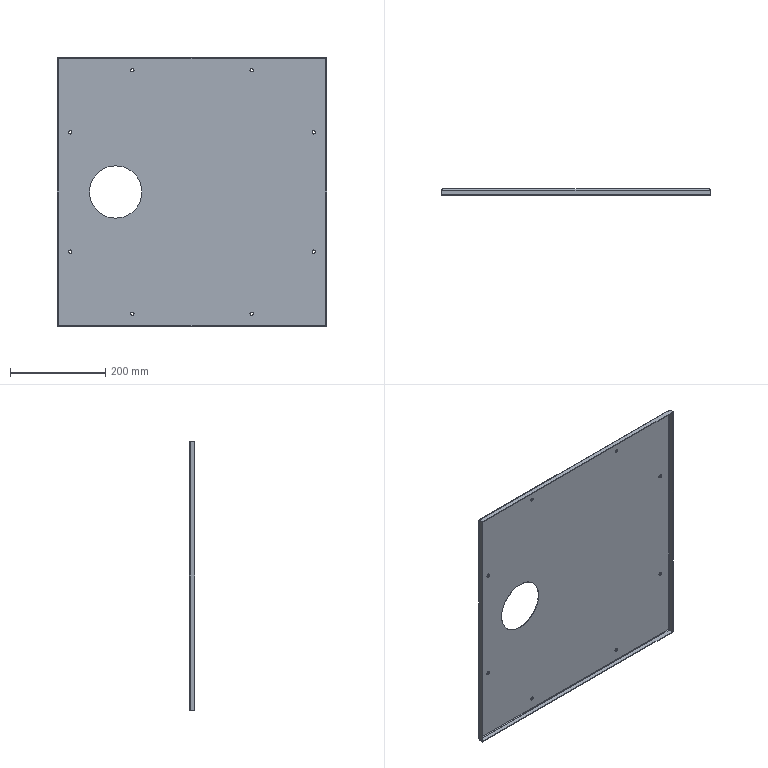Part | STEP file | 1 solid | 64 faces | box 565 x 12 x 565 mm | volume 496282 mm3 | plane 38 | cylinder 26 | commonest cylinder face diameters 7 x16 3 x4 6 x4 110 x2